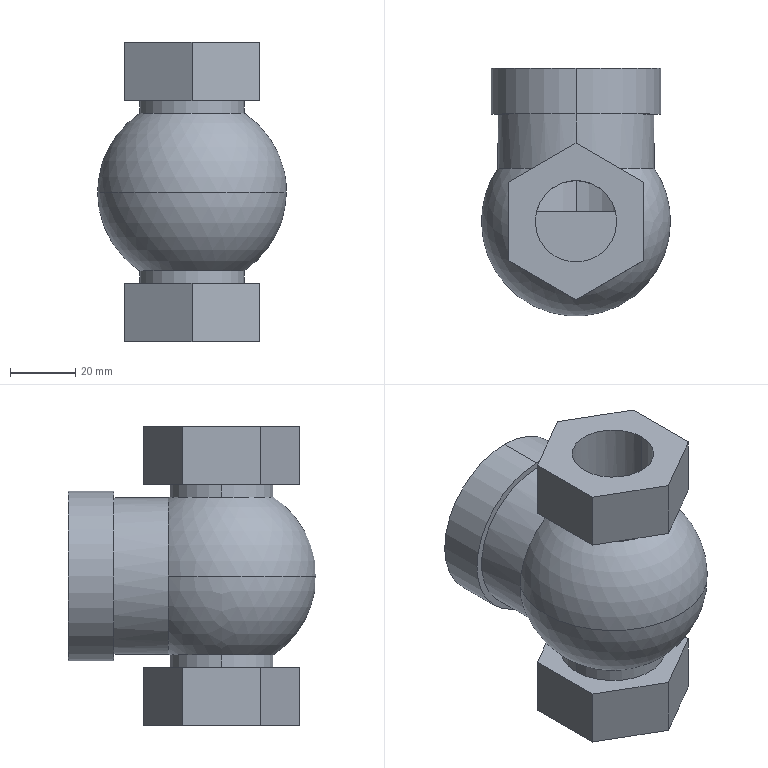Part | SolidWorks | features ICE 8, RevCut 3, MirrorPattern 1, Revolution 1 | 1 solid | 49 faces | box 58 x 76 x 92 mm | volume 132810 mm3 | plane 23 | cylinder 22 | sphere 2 | cone 2 | commonest cylinder face diameters 5 x6 25 x4 32 x4 35 x2 40 x2 48 x2
STEP:
#1=CARTESIAN_POINT('',(0.,-1.,2.5));
#2=VERTEX_POINT('',#1);
#3=CARTESIAN_POINT('',(0.,-1.,-2.5));
#4=VERTEX_POINT('',#3);
#5=CARTESIAN_POINT('',(0.,-1.,0.));
#6=DIRECTION('',(0.,-1.,0.));
#7=DIRECTION('',(0.,0.,1.));
#8=AXIS2_PLACEMENT_3D('',#5,#6,#7);
#9=CIRCLE('',#8,2.5);
#10=EDGE_CURVE('',#2,#4,#9,.T.);
#11=ORIENTED_EDGE('',*,*,#10,.F.);
#12=CARTESIAN_POINT('',(0.,-2.5,2.5));
#13=VERTEX_POINT('',#12);
#14=CARTESIAN_POINT('',(0.,-5.,2.5));
#15=DIRECTION('',(0.,-1.,0.));
#16=VECTOR('',#15,1000.);
#17=LINE('',#14,#16);
#18=EDGE_CURVE('',#2,#13,#17,.T.);
#19=ORIENTED_EDGE('',*,*,#18,.T.);
#20=CARTESIAN_POINT('',(-2.5,-5.,0.));
#21=VERTEX_POINT('',#20);
#22=CARTESIAN_POINT('',(0.,-2.5,2.5));
#23=CARTESIAN_POINT('',(-1.464,-2.5,2.5));
#24=CARTESIAN_POINT('',(-2.5,-3.536,1.464));
#25=CARTESIAN_POINT('',(-2.5,-5.,0.));
#26=(BOUNDED_CURVE()B_SPLINE_CURVE(3,(#22,#23,#24,#25),.UNSPECIFIED.,.F.,.T.)B_SPLINE_CURVE_WITH_KNOTS((4,4),(0.,1.571),.UNSPECIFIED.)CURVE()GEOMETRIC_REPRESENTATION_ITEM()RATIONAL_B_SPLINE_CURVE((1.,0.8047,0.8047,1.))REPRESENTATION_ITEM(''));
#27=EDGE_CURVE('',#13,#21,#26,.T.);
#28=ORIENTED_EDGE('',*,*,#27,.T.);
#29=CARTESIAN_POINT('',(0.,-2.5,-2.5));
#30=VERTEX_POINT('',#29);
#31=CARTESIAN_POINT('',(-2.5,-5.,0.));
#32=CARTESIAN_POINT('',(-2.5,-3.536,-1.464));
#33=CARTESIAN_POINT('',(-1.464,-2.5,-2.5));
#34=CARTESIAN_POINT('',(0.,-2.5,-2.5));
#35=(BOUNDED_CURVE()B_SPLINE_CURVE(3,(#31,#32,#33,#34),.UNSPECIFIED.,.F.,.T.)B_SPLINE_CURVE_WITH_KNOTS((4,4),(1.571,3.142),.UNSPECIFIED.)CURVE()GEOMETRIC_REPRESENTATION_ITEM()RATIONAL_B_SPLINE_CURVE((1.,0.8047,0.8047,1.))REPRESENTATION_ITEM(''));
#36=EDGE_CURVE('',#21,#30,#35,.T.);
#37=ORIENTED_EDGE('',*,*,#36,.T.);
#38=CARTESIAN_POINT('',(0.,-5.,-2.5));
#39=DIRECTION('',(0.,-1.,0.));
#40=VECTOR('',#39,1000.);
#41=LINE('',#38,#40);
#42=EDGE_CURVE('',#4,#30,#41,.T.);
#43=ORIENTED_EDGE('',*,*,#42,.F.);
#44=EDGE_LOOP('',(#11,#19,#28,#37,#43));
#45=FACE_OUTER_BOUND('',#44,.T.);
#46=CARTESIAN_POINT('',(0.,-5.,0.));
#47=DIRECTION('',(0.,-1.,0.));
#48=DIRECTION('',(0.,0.,-1.));
#49=AXIS2_PLACEMENT_3D('',#46,#47,#48);
#50=CYLINDRICAL_SURFACE('',#49,2.5);
#51=ADVANCED_FACE('',(#45),#50,.F.);
#52=CARTESIAN_POINT('',(0.,3.,-17.5));
#53=VERTEX_POINT('',#52);
#54=CARTESIAN_POINT('',(-12.135,3.,12.61));
#55=VERTEX_POINT('',#54);
#56=CARTESIAN_POINT('',(0.,3.,0.));
#57=DIRECTION('',(0.,1.,0.));
#58=DIRECTION('',(0.,0.,1.));
#59=AXIS2_PLACEMENT_3D('',#56,#57,#58);
#60=CIRCLE('',#59,17.5);
#61=EDGE_CURVE('',#53,#55,#60,.T.);
#62=ORIENTED_EDGE('',*,*,#61,.F.);
#63=CARTESIAN_POINT('',(0.,42.,-17.5));
#64=VERTEX_POINT('',#63);
#65=CARTESIAN_POINT('',(0.,3.,-17.5));
#66=DIRECTION('',(0.,1.,0.));
#67=VECTOR('',#66,1000.);
#68=LINE('',#65,#67);
#69=EDGE_CURVE('',#53,#64,#68,.T.);
#70=ORIENTED_EDGE('',*,*,#69,.T.);
#71=CARTESIAN_POINT('',(0.,42.,17.5));
#72=VERTEX_POINT('',#71);
#73=CARTESIAN_POINT('',(0.,42.,0.));
#74=DIRECTION('',(0.,1.,0.));
#75=DIRECTION('',(0.,0.,1.));
#76=AXIS2_PLACEMENT_3D('',#73,#74,#75);
#77=CIRCLE('',#76,17.5);
#78=EDGE_CURVE('',#64,#72,#77,.T.);
#79=ORIENTED_EDGE('',*,*,#78,.T.);
#80=CARTESIAN_POINT('',(0.,12.5,17.5));
#81=VERTEX_POINT('',#80);
#82=CARTESIAN_POINT('',(0.,3.,17.5));
#83=DIRECTION('',(0.,1.,0.));
#84=VECTOR('',#83,1000.);
#85=LINE('',#82,#84);
#86=EDGE_CURVE('',#81,#72,#85,.T.);
#87=ORIENTED_EDGE('',*,*,#86,.F.);
#88=CARTESIAN_POINT('',(-12.135,3.,12.61));
#89=CARTESIAN_POINT('',(-11.963,3.695,12.775));
#90=CARTESIAN_POINT('',(-11.738,4.351,12.984));
#91=CARTESIAN_POINT('',(-11.195,5.602,13.455));
#92=CARTESIAN_POINT('',(-10.877,6.198,13.717));
#93=CARTESIAN_POINT('',(-10.143,7.337,14.268));
#94=CARTESIAN_POINT('',(-9.736,7.868,14.551));
#95=CARTESIAN_POINT('',(-8.842,8.86,15.111));
#96=CARTESIAN_POINT('',(-8.356,9.322,15.388));
#97=CARTESIAN_POINT('',(-7.293,10.175,15.919));
#98=CARTESIAN_POINT('',(-6.728,10.557,16.167));
#99=CARTESIAN_POINT('',(-5.537,11.228,16.613));
#100=CARTESIAN_POINT('',(-4.909,11.518,16.811));
#101=CARTESIAN_POINT('',(-3.911,11.878,17.061));
#102=CARTESIAN_POINT('',(-3.567,11.986,17.136));
#103=CARTESIAN_POINT('',(-2.872,12.171,17.266));
#104=CARTESIAN_POINT('',(-2.522,12.248,17.321));
#105=CARTESIAN_POINT('',(-1.813,12.373,17.409));
#106=CARTESIAN_POINT('',(-1.455,12.42,17.443));
#107=CARTESIAN_POINT('',(-0.733,12.484,17.488));
#108=CARTESIAN_POINT('',(-0.3665,12.5,17.5));
#109=CARTESIAN_POINT('',(0.,12.5,17.5));
#110=B_SPLINE_CURVE_WITH_KNOTS('',3,(#88,#89,#90,#91,#92,#93,#94,#95,#96,#97,#98,#99,#100,#101,#102,#103,#104,#105,#106,#107,#108,#109),.UNSPECIFIED.,.F.,.F.,(4,2,2,2,2,2,2,2,2,2,4),(0.,0.002165,0.00433,0.006494,0.008659,0.01082,0.01299,0.01407,0.01515,0.01624,0.01732),.UNSPECIFIED.);
#111=EDGE_CURVE('',#55,#81,#110,.T.);
#112=ORIENTED_EDGE('',*,*,#111,.F.);
#113=EDGE_LOOP('',(#62,#70,#79,#87,#112));
#114=FACE_OUTER_BOUND('',#113,.T.);
#115=CARTESIAN_POINT('',(0.,3.,0.));
#116=DIRECTION('',(0.,1.,0.));
#117=DIRECTION('',(0.,0.,1.));
#118=AXIS2_PLACEMENT_3D('',#115,#116,#117);
#119=CYLINDRICAL_SURFACE('',#118,17.5);
#120=ADVANCED_FACE('',(#114),#119,.F.);
#121=CARTESIAN_POINT('',(12.5,0.,-21.));
#122=VERTEX_POINT('',#121);
#123=CARTESIAN_POINT('',(-12.5,0.,-21.));
#124=VERTEX_POINT('',#123);
#125=CARTESIAN_POINT('',(0.,0.,-21.));
#126=DIRECTION('',(0.,0.,-1.));
#127=DIRECTION('',(-1.,0.,0.));
#128=AXIS2_PLACEMENT_3D('',#125,#126,#127);
#129=CIRCLE('',#128,12.5);
#130=EDGE_CURVE('',#122,#124,#129,.T.);
#131=ORIENTED_EDGE('',*,*,#130,.F.);
#132=CARTESIAN_POINT('',(12.5,0.,-46.));
#133=VERTEX_POINT('',#132);
#134=CARTESIAN_POINT('',(12.5,0.,-21.));
#135=DIRECTION('',(0.,0.,-1.));
#136=VECTOR('',#135,1000.);
#137=LINE('',#134,#136);
#138=EDGE_CURVE('',#122,#133,#137,.T.);
#139=ORIENTED_EDGE('',*,*,#138,.T.);
#140=CARTESIAN_POINT('',(-12.5,0.,-46.));
#141=VERTEX_POINT('',#140);
#142=CARTESIAN_POINT('',(0.,0.,-46.));
#143=DIRECTION('',(0.,0.,-1.));
#144=DIRECTION('',(-1.,0.,0.));
#145=AXIS2_PLACEMENT_3D('',#142,#143,#144);
#146=CIRCLE('',#145,12.5);
#147=EDGE_CURVE('',#133,#141,#146,.T.);
#148=ORIENTED_EDGE('',*,*,#147,.T.);
#149=CARTESIAN_POINT('',(-12.5,0.,-21.));
#150=DIRECTION('',(0.,0.,-1.));
#151=VECTOR('',#150,1000.);
#152=LINE('',#149,#151);
#153=EDGE_CURVE('',#124,#141,#152,.T.);
#154=ORIENTED_EDGE('',*,*,#153,.F.);
#155=EDGE_LOOP('',(#131,#139,#148,#154));
#156=FACE_OUTER_BOUND('',#155,.T.);
#157=CARTESIAN_POINT('',(0.,0.,-21.));
#158=DIRECTION('',(0.,0.,-1.));
#159=DIRECTION('',(-1.,0.,0.));
#160=AXIS2_PLACEMENT_3D('',#157,#158,#159);
#161=CYLINDRICAL_SURFACE('',#160,12.5);
#162=ADVANCED_FACE('',(#156),#161,.F.);
#163=CARTESIAN_POINT('',(0.,42.,-20.));
#164=VERTEX_POINT('',#163);
#165=CARTESIAN_POINT('',(0.,42.,20.));
#166=VERTEX_POINT('',#165);
#167=CARTESIAN_POINT('',(0.,42.,0.));
#168=DIRECTION('',(0.,1.,0.));
#169=DIRECTION('',(0.,0.,1.));
#170=AXIS2_PLACEMENT_3D('',#167,#168,#169);
#171=CIRCLE('',#170,20.);
#172=EDGE_CURVE('',#164,#166,#171,.T.);
#173=ORIENTED_EDGE('',*,*,#172,.F.);
#174=CARTESIAN_POINT('',(0.,47.,-20.));
#175=VERTEX_POINT('',#174);
#176=CARTESIAN_POINT('',(0.,42.,-20.));
#177=DIRECTION('',(0.,1.,0.));
#178=VECTOR('',#177,1000.);
#179=LINE('',#176,#178);
#180=EDGE_CURVE('',#164,#175,#179,.T.);
#181=ORIENTED_EDGE('',*,*,#180,.T.);
#182=CARTESIAN_POINT('',(0.,47.,20.));
#183=VERTEX_POINT('',#182);
#184=CARTESIAN_POINT('',(0.,47.,0.));
#185=DIRECTION('',(0.,1.,0.));
#186=DIRECTION('',(0.,0.,1.));
#187=AXIS2_PLACEMENT_3D('',#184,#185,#186);
#188=CIRCLE('',#187,20.);
#189=EDGE_CURVE('',#175,#183,#188,.T.);
#190=ORIENTED_EDGE('',*,*,#189,.T.);
#191=CARTESIAN_POINT('',(0.,42.,20.));
#192=DIRECTION('',(0.,1.,0.));
#193=VECTOR('',#192,1000.);
#194=LINE('',#191,#193);
#195=EDGE_CURVE('',#166,#183,#194,.T.);
#196=ORIENTED_EDGE('',*,*,#195,.F.);
#197=EDGE_LOOP('',(#173,#181,#190,#196));
#198=FACE_OUTER_BOUND('',#197,.T.);
#199=CARTESIAN_POINT('',(0.,42.,0.));
#200=DIRECTION('',(0.,1.,0.));
#201=DIRECTION('',(0.,0.,1.));
#202=AXIS2_PLACEMENT_3D('',#199,#200,#201);
#203=CYLINDRICAL_SURFACE('',#202,20.);
#204=ADVANCED_FACE('',(#198),#203,.F.);
#205=CARTESIAN_POINT('',(0.,33.,26.));
#206=VERTEX_POINT('',#205);
#207=CARTESIAN_POINT('',(0.,33.,-26.));
#208=VERTEX_POINT('',#207);
#209=CARTESIAN_POINT('',(0.,33.,0.));
#210=DIRECTION('',(0.,1.,0.));
#211=DIRECTION('',(0.,0.,1.));
#212=AXIS2_PLACEMENT_3D('',#209,#210,#211);
#213=CIRCLE('',#212,26.);
#214=EDGE_CURVE('',#206,#208,#213,.T.);
#215=ORIENTED_EDGE('',*,*,#214,.T.);
#216=CARTESIAN_POINT('',(0.,47.,-26.));
#217=VERTEX_POINT('',#216);
#218=CARTESIAN_POINT('',(0.,33.,-26.));
#219=DIRECTION('',(0.,1.,0.));
#220=VECTOR('',#219,1000.);
#221=LINE('',#218,#220);
#222=EDGE_CURVE('',#208,#217,#221,.T.);
#223=ORIENTED_EDGE('',*,*,#222,.T.);
#224=CARTESIAN_POINT('',(0.,47.,26.));
#225=VERTEX_POINT('',#224);
#226=CARTESIAN_POINT('',(0.,47.,0.));
#227=DIRECTION('',(0.,1.,0.));
#228=DIRECTION('',(0.,0.,1.));
#229=AXIS2_PLACEMENT_3D('',#226,#227,#228);
#230=CIRCLE('',#229,26.);
#231=EDGE_CURVE('',#225,#217,#230,.T.);
#232=ORIENTED_EDGE('',*,*,#231,.F.);
#233=CARTESIAN_POINT('',(0.,33.,26.));
#234=DIRECTION('',(0.,1.,0.));
#235=VECTOR('',#234,1000.);
#236=LINE('',#233,#235);
#237=EDGE_CURVE('',#206,#225,#236,.T.);
#238=ORIENTED_EDGE('',*,*,#237,.F.);
#239=EDGE_LOOP('',(#215,#223,#232,#238));
#240=FACE_OUTER_BOUND('',#239,.T.);
#241=CARTESIAN_POINT('',(0.,33.,0.));
#242=DIRECTION('',(0.,1.,0.));
#243=DIRECTION('',(0.,0.,1.));
#244=AXIS2_PLACEMENT_3D('',#241,#242,#243);
#245=CYLINDRICAL_SURFACE('',#244,26.);
#246=ADVANCED_FACE('',(#240),#245,.T.);
#247=CARTESIAN_POINT('',(0.,33.,24.));
#248=VERTEX_POINT('',#247);
#249=CARTESIAN_POINT('',(0.,33.,-24.));
#250=VERTEX_POINT('',#249);
#251=CARTESIAN_POINT('',(0.,33.,0.));
#252=DIRECTION('',(0.,1.,0.));
#253=DIRECTION('',(0.,0.,1.));
#254=AXIS2_PLACEMENT_3D('',#251,#252,#253);
#255=CIRCLE('',#254,24.);
#256=EDGE_CURVE('',#248,#250,#255,.T.);
#257=ORIENTED_EDGE('',*,*,#256,.F.);
#258=CARTESIAN_POINT('',(0.,16.279,24.));
#259=VERTEX_POINT('',#258);
#260=CARTESIAN_POINT('',(0.,47.,24.));
#261=DIRECTION('',(0.,-1.,0.));
#262=VECTOR('',#261,1000.);
#263=LINE('',#260,#262);
#264=EDGE_CURVE('',#248,#259,#263,.T.);
#265=ORIENTED_EDGE('',*,*,#264,.T.);
#266=CARTESIAN_POINT('',(24.,16.279,0.));
#267=VERTEX_POINT('',#266);
#268=CARTESIAN_POINT('',(0.,16.279,0.));
#269=DIRECTION('',(0.,1.,0.));
#270=DIRECTION('',(0.,0.,-1.));
#271=AXIS2_PLACEMENT_3D('',#268,#269,#270);
#272=CIRCLE('',#271,24.);
#273=EDGE_CURVE('',#259,#267,#272,.T.);
#274=ORIENTED_EDGE('',*,*,#273,.T.);
#275=CARTESIAN_POINT('',(0.,16.279,-24.));
#276=VERTEX_POINT('',#275);
#277=CARTESIAN_POINT('',(0.,16.279,0.));
#278=DIRECTION('',(0.,1.,0.));
#279=DIRECTION('',(0.,0.,-1.));
#280=AXIS2_PLACEMENT_3D('',#277,#278,#279);
#281=CIRCLE('',#280,24.);
#282=EDGE_CURVE('',#267,#276,#281,.T.);
#283=ORIENTED_EDGE('',*,*,#282,.T.);
#284=CARTESIAN_POINT('',(0.,47.,-24.));
#285=DIRECTION('',(0.,-1.,0.));
#286=VECTOR('',#285,1000.);
#287=LINE('',#284,#286);
#288=EDGE_CURVE('',#250,#276,#287,.T.);
#289=ORIENTED_EDGE('',*,*,#288,.F.);
#290=EDGE_LOOP('',(#257,#265,#274,#283,#289));
#291=FACE_OUTER_BOUND('',#290,.T.);
#292=CARTESIAN_POINT('',(0.,47.,0.));
#293=DIRECTION('',(0.,-1.,0.));
#294=DIRECTION('',(0.,0.,-1.));
#295=AXIS2_PLACEMENT_3D('',#292,#293,#294);
#296=CYLINDRICAL_SURFACE('',#295,24.);
#297=ADVANCED_FACE('',(#291),#296,.T.);
#298=CARTESIAN_POINT('',(16.,0.,-24.187));
#299=VERTEX_POINT('',#298);
#300=CARTESIAN_POINT('',(-16.,0.,-24.187));
#301=VERTEX_POINT('',#300);
#302=CARTESIAN_POINT('',(0.,0.,-24.187));
#303=DIRECTION('',(0.,0.,1.));
#304=DIRECTION('',(1.,0.,0.));
#305=AXIS2_PLACEMENT_3D('',#302,#303,#304);
#306=CIRCLE('',#305,16.);
#307=EDGE_CURVE('',#299,#301,#306,.T.);
#308=ORIENTED_EDGE('',*,*,#307,.T.);
#309=CARTESIAN_POINT('',(0.,0.,-24.187));
#310=DIRECTION('',(0.,0.,1.));
#311=DIRECTION('',(1.,0.,0.));
#312=AXIS2_PLACEMENT_3D('',#309,#310,#311);
#313=CIRCLE('',#312,16.);
#314=EDGE_CURVE('',#301,#299,#313,.T.);
#315=ORIENTED_EDGE('',*,*,#314,.T.);
#316=EDGE_LOOP('',(#308,#315));
#317=FACE_BOUND('',#316,.T.);
#318=CARTESIAN_POINT('',(29.,0.,0.));
#319=VERTEX_POINT('',#318);
#320=CARTESIAN_POINT('',(0.,0.,0.));
#321=DIRECTION('',(0.,0.,1.));
#322=DIRECTION('',(1.,0.,0.));
#323=AXIS2_PLACEMENT_3D('',#320,#321,#322);
#324=CIRCLE('',#323,29.);
#325=EDGE_CURVE('',#319,#267,#324,.T.);
#326=ORIENTED_EDGE('',*,*,#325,.F.);
#327=CARTESIAN_POINT('',(-29.,0.,0.));
#328=VERTEX_POINT('',#327);
#329=CARTESIAN_POINT('',(0.,0.,0.));
#330=DIRECTION('',(0.,0.,-1.));
#331=DIRECTION('',(0.,1.,0.));
#332=AXIS2_PLACEMENT_3D('',#329,#330,#331);
#333=CIRCLE('',#332,29.);
#334=EDGE_CURVE('',#319,#328,#333,.T.);
#335=ORIENTED_EDGE('',*,*,#334,.T.);
#336=CARTESIAN_POINT('',(-24.,16.279,0.));
#337=VERTEX_POINT('',#336);
#338=CARTESIAN_POINT('',(0.,0.,0.));
#339=DIRECTION('',(0.,0.,1.));
#340=DIRECTION('',(1.,0.,0.));
#341=AXIS2_PLACEMENT_3D('',#338,#339,#340);
#342=CIRCLE('',#341,29.);
#343=EDGE_CURVE('',#337,#328,#342,.T.);
#344=ORIENTED_EDGE('',*,*,#343,.F.);
#345=CARTESIAN_POINT('',(0.,16.279,0.));
#346=DIRECTION('',(0.,1.,0.));
#347=DIRECTION('',(0.,0.,-1.));
#348=AXIS2_PLACEMENT_3D('',#345,#346,#347);
#349=CIRCLE('',#348,24.);
#350=EDGE_CURVE('',#276,#337,#349,.T.);
#351=ORIENTED_EDGE('',*,*,#350,.F.);
#352=ORIENTED_EDGE('',*,*,#282,.F.);
#353=EDGE_LOOP('',(#326,#335,#344,#351,#352));
#354=FACE_OUTER_BOUND('',#353,.T.);
#355=CARTESIAN_POINT('',(0.,0.,0.));
#356=DIRECTION('',(0.,0.,-1.));
#357=DIRECTION('',(0.,1.,0.));
#358=AXIS2_PLACEMENT_3D('',#355,#356,#357);
#359=SPHERICAL_SURFACE('',#358,29.);
#360=ADVANCED_FACE('',(#317,#354),#359,.T.);
#361=CARTESIAN_POINT('',(16.,0.,28.));
#362=VERTEX_POINT('',#361);
#363=CARTESIAN_POINT('',(-16.,0.,28.));
#364=VERTEX_POINT('',#363);
#365=CARTESIAN_POINT('',(0.,0.,28.));
#366=DIRECTION('',(0.,0.,1.));
#367=DIRECTION('',(1.,0.,0.));
#368=AXIS2_PLACEMENT_3D('',#365,#366,#367);
#369=CIRCLE('',#368,16.);
#370=EDGE_CURVE('',#362,#364,#369,.T.);
#371=ORIENTED_EDGE('',*,*,#370,.F.);
#372=CARTESIAN_POINT('',(16.,0.,24.187));
#373=VERTEX_POINT('',#372);
#374=CARTESIAN_POINT('',(16.,0.,46.));
#375=DIRECTION('',(0.,0.,-1.));
#376=VECTOR('',#375,1000.);
#377=LINE('',#374,#376);
#378=EDGE_CURVE('',#362,#373,#377,.T.);
#379=ORIENTED_EDGE('',*,*,#378,.T.);
#380=CARTESIAN_POINT('',(-16.,0.,24.187));
#381=VERTEX_POINT('',#380);
#382=CARTESIAN_POINT('',(0.,0.,24.187));
#383=DIRECTION('',(0.,0.,1.));
#384=DIRECTION('',(-1.,0.,0.));
#385=AXIS2_PLACEMENT_3D('',#382,#383,#384);
#386=CIRCLE('',#385,16.);
#387=EDGE_CURVE('',#373,#381,#386,.T.);
#388=ORIENTED_EDGE('',*,*,#387,.T.);
#389=CARTESIAN_POINT('',(-16.,0.,46.));
#390=DIRECTION('',(0.,0.,-1.));
#391=VECTOR('',#390,1000.);
#392=LINE('',#389,#391);
#393=EDGE_CURVE('',#364,#381,#392,.T.);
#394=ORIENTED_EDGE('',*,*,#393,.F.);
#395=EDGE_LOOP('',(#371,#379,#388,#394));
#396=FACE_OUTER_BOUND('',#395,.T.);
#397=CARTESIAN_POINT('',(0.,0.,46.));
#398=DIRECTION('',(0.,0.,-1.));
#399=DIRECTION('',(-1.,0.,0.));
#400=AXIS2_PLACEMENT_3D('',#397,#398,#399);
#401=CYLINDRICAL_SURFACE('',#400,16.);
#402=ADVANCED_FACE('',(#396),#401,.T.);
#403=CARTESIAN_POINT('',(16.,0.,-28.));
#404=VERTEX_POINT('',#403);
#405=CARTESIAN_POINT('',(-16.,0.,-28.));
#406=VERTEX_POINT('',#405);
#407=CARTESIAN_POINT('',(0.,0.,-28.));
#408=DIRECTION('',(0.,0.,1.));
#409=DIRECTION('',(-1.,0.,0.));
#410=AXIS2_PLACEMENT_3D('',#407,#408,#409);
#411=CIRCLE('',#410,16.);
#412=EDGE_CURVE('',#404,#406,#411,.T.);
#413=ORIENTED_EDGE('',*,*,#412,.T.);
#414=CARTESIAN_POINT('',(-16.,0.,-46.));
#415=DIRECTION('',(0.,0.,1.));
#416=VECTOR('',#415,1000.);
#417=LINE('',#414,#416);
#418=EDGE_CURVE('',#406,#301,#417,.T.);
#419=ORIENTED_EDGE('',*,*,#418,.T.);
#420=ORIENTED_EDGE('',*,*,#307,.F.);
#421=CARTESIAN_POINT('',(16.,0.,-46.));
#422=DIRECTION('',(0.,0.,1.));
#423=VECTOR('',#422,1000.);
#424=LINE('',#421,#423);
#425=EDGE_CURVE('',#404,#299,#424,.T.);
#426=ORIENTED_EDGE('',*,*,#425,.F.);
#427=EDGE_LOOP('',(#413,#419,#420,#426));
#428=FACE_OUTER_BOUND('',#427,.T.);
#429=CARTESIAN_POINT('',(0.,0.,-46.));
#430=DIRECTION('',(0.,0.,1.));
#431=DIRECTION('',(1.,0.,0.));
#432=AXIS2_PLACEMENT_3D('',#429,#430,#431);
#433=CYLINDRICAL_SURFACE('',#432,16.);
#434=ADVANCED_FACE('',(#428),#433,.T.);
#435=CARTESIAN_POINT('',(-12.5,0.,12.));
#436=VERTEX_POINT('',#435);
#437=CARTESIAN_POINT('',(12.5,0.,12.));
#438=VERTEX_POINT('',#437);
#439=CARTESIAN_POINT('',(0.,0.,12.));
#440=DIRECTION('',(0.,0.,1.));
#441=DIRECTION('',(1.,0.,0.));
#442=AXIS2_PLACEMENT_3D('',#439,#440,#441);
#443=CIRCLE('',#442,12.5);
#444=EDGE_CURVE('',#436,#438,#443,.T.);
#445=ORIENTED_EDGE('',*,*,#444,.F.);
#446=CARTESIAN_POINT('',(-12.5,0.,46.));
#447=VERTEX_POINT('',#446);
#448=CARTESIAN_POINT('',(-12.5,0.,12.));
#449=DIRECTION('',(0.,0.,1.));
#450=VECTOR('',#449,1000.);
#451=LINE('',#448,#450);
#452=EDGE_CURVE('',#436,#447,#451,.T.);
#453=ORIENTED_EDGE('',*,*,#452,.T.);
#454=CARTESIAN_POINT('',(12.5,0.,46.));
#455=VERTEX_POINT('',#454);
#456=CARTESIAN_POINT('',(0.,0.,46.));
#457=DIRECTION('',(0.,0.,1.));
#458=DIRECTION('',(1.,0.,0.));
#459=AXIS2_PLACEMENT_3D('',#456,#457,#458);
#460=CIRCLE('',#459,12.5);
#461=EDGE_CURVE('',#447,#455,#460,.T.);
#462=ORIENTED_EDGE('',*,*,#461,.T.);
#463=CARTESIAN_POINT('',(12.5,0.,12.));
#464=DIRECTION('',(0.,0.,1.));
#465=VECTOR('',#464,1000.);
#466=LINE('',#463,#465);
#467=EDGE_CURVE('',#438,#455,#466,.T.);
#468=ORIENTED_EDGE('',*,*,#467,.F.);
#469=EDGE_LOOP('',(#445,#453,#462,#468));
#470=FACE_OUTER_BOUND('',#469,.T.);
#471=CARTESIAN_POINT('',(0.,0.,12.));
#472=DIRECTION('',(0.,0.,1.));
#473=DIRECTION('',(1.,0.,0.));
#474=AXIS2_PLACEMENT_3D('',#471,#472,#473);
#475=CYLINDRICAL_SURFACE('',#474,12.5);
#476=ADVANCED_FACE('',(#470),#475,.F.);
#477=CARTESIAN_POINT('',(2.5,-5.,-21.));
#478=VERTEX_POINT('',#477);
#479=CARTESIAN_POINT('',(-2.5,-5.,-21.));
#480=VERTEX_POINT('',#479);
#481=CARTESIAN_POINT('',(0.,-5.,-21.));
#482=DIRECTION('',(0.,0.,-1.));
#483=DIRECTION('',(-1.,0.,0.));
#484=AXIS2_PLACEMENT_3D('',#481,#482,#483);
#485=CIRCLE('',#484,2.5);
#486=EDGE_CURVE('',#478,#480,#485,.T.);
#487=ORIENTED_EDGE('',*,*,#486,.T.);
#488=CARTESIAN_POINT('',(-2.5,-5.,4.897));
#489=DIRECTION('',(0.,0.,1.));
#490=VECTOR('',#489,1000.);
#491=LINE('',#488,#490);
#492=EDGE_CURVE('',#480,#21,#491,.T.);
#493=ORIENTED_EDGE('',*,*,#492,.T.);
#494=CARTESIAN_POINT('',(-2.5,-5.,2.5));
#495=VERTEX_POINT('',#494);
#496=CARTESIAN_POINT('',(-2.5,-5.,4.897));
#497=DIRECTION('',(0.,0.,1.));
#498=VECTOR('',#497,1000.);
#499=LINE('',#496,#498);
#500=EDGE_CURVE('',#21,#495,#499,.T.);
#501=ORIENTED_EDGE('',*,*,#500,.T.);
#502=CARTESIAN_POINT('',(2.5,-5.,2.5));
#503=VERTEX_POINT('',#502);
#504=CARTESIAN_POINT('',(0.,-5.,2.5));
#505=DIRECTION('',(0.,0.,1.));
#506=DIRECTION('',(1.,0.,0.));
#507=AXIS2_PLACEMENT_3D('',#504,#505,#506);
#508=CIRCLE('',#507,2.5);
#509=EDGE_CURVE('',#495,#503,#508,.T.);
#510=ORIENTED_EDGE('',*,*,#509,.T.);
#511=CARTESIAN_POINT('',(2.5,-5.,0.));
#512=VERTEX_POINT('',#511);
#513=CARTESIAN_POINT('',(2.5,-5.,4.897));
#514=DIRECTION('',(0.,0.,1.));
#515=VECTOR('',#514,1000.);
#516=LINE('',#513,#515);
#517=EDGE_CURVE('',#512,#503,#516,.T.);
#518=ORIENTED_EDGE('',*,*,#517,.F.);
#519=CARTESIAN_POINT('',(2.5,-5.,4.897));
#520=DIRECTION('',(0.,0.,1.));
#521=VECTOR('',#520,1000.);
#522=LINE('',#519,#521);
#523=EDGE_CURVE('',#478,#512,#522,.T.);
#524=ORIENTED_EDGE('',*,*,#523,.F.);
#525=EDGE_LOOP('',(#487,#493,#501,#510,#518,#524));
#526=FACE_OUTER_BOUND('',#525,.T.);
#527=CARTESIAN_POINT('',(0.,-5.,4.897));
#528=DIRECTION('',(0.,0.,1.));
#529=DIRECTION('',(1.,0.,0.));
#530=AXIS2_PLACEMENT_3D('',#527,#528,#529);
#531=CYLINDRICAL_SURFACE('',#530,2.5);
#532=ADVANCED_FACE('',(#526),#531,.F.);
#533=ORIENTED_EDGE('',*,*,#492,.F.);
#534=CARTESIAN_POINT('',(0.,-5.,-21.));
#535=DIRECTION('',(0.,0.,-1.));
#536=DIRECTION('',(-1.,0.,0.));
#537=AXIS2_PLACEMENT_3D('',#534,#535,#536);
#538=CIRCLE('',#537,2.5);
#539=EDGE_CURVE('',#480,#478,#538,.T.);
#540=ORIENTED_EDGE('',*,*,#539,.T.);
#541=ORIENTED_EDGE('',*,*,#523,.T.);
#542=CARTESIAN_POINT('',(0.,-2.5,-2.5));
#543=CARTESIAN_POINT('',(1.464,-2.5,-2.5));
#544=CARTESIAN_POINT('',(2.5,-3.536,-1.464));
#545=CARTESIAN_POINT('',(2.5,-5.,0.));
#546=(BOUNDED_CURVE()B_SPLINE_CURVE(3,(#542,#543,#544,#545),.UNSPECIFIED.,.F.,.T.)B_SPLINE_CURVE_WITH_KNOTS((4,4),(3.142,4.712),.UNSPECIFIED.)CURVE()GEOMETRIC_REPRESENTATION_ITEM()RATIONAL_B_SPLINE_CURVE((1.,0.8047,0.8047,1.))REPRESENTATION_ITEM(''));
#547=EDGE_CURVE('',#30,#512,#546,.T.);
#548=ORIENTED_EDGE('',*,*,#547,.F.);
#549=ORIENTED_EDGE('',*,*,#36,.F.);
#550=EDGE_LOOP('',(#533,#540,#541,#548,#549));
#551=FACE_OUTER_BOUND('',#550,.T.);
#552=CARTESIAN_POINT('',(0.,-5.,4.897));
#553=DIRECTION('',(0.,0.,1.));
#554=DIRECTION('',(1.,0.,0.));
#555=AXIS2_PLACEMENT_3D('',#552,#553,#554);
#556=CYLINDRICAL_SURFACE('',#555,2.5);
#557=ADVANCED_FACE('',(#551),#556,.F.);
#558=CARTESIAN_POINT('',(2.5,-5.,0.));
#559=CARTESIAN_POINT('',(2.5,-3.536,1.464));
#560=CARTESIAN_POINT('',(1.464,-2.5,2.5));
#561=CARTESIAN_POINT('',(0.,-2.5,2.5));
#562=(BOUNDED_CURVE()B_SPLINE_CURVE(3,(#558,#559,#560,#561),.UNSPECIFIED.,.F.,.T.)B_SPLINE_CURVE_WITH_KNOTS((4,4),(4.712,6.283),.UNSPECIFIED.)CURVE()GEOMETRIC_REPRESENTATION_ITEM()RATIONAL_B_SPLINE_CURVE((1.,0.8047,0.8047,1.))REPRESENTATION_ITEM(''));
#563=EDGE_CURVE('',#512,#13,#562,.T.);
#564=ORIENTED_EDGE('',*,*,#563,.F.);
#565=ORIENTED_EDGE('',*,*,#517,.T.);
#566=CARTESIAN_POINT('',(0.,-5.,2.5));
#567=DIRECTION('',(0.,0.,1.));
#568=DIRECTION('',(1.,0.,0.));
#569=AXIS2_PLACEMENT_3D('',#566,#567,#568);
#570=CIRCLE('',#569,2.5);
#571=EDGE_CURVE('',#503,#13,#570,.T.);
#572=ORIENTED_EDGE('',*,*,#571,.T.);
#573=EDGE_LOOP('',(#564,#565,#572));
#574=FACE_OUTER_BOUND('',#573,.T.);
#575=CARTESIAN_POINT('',(0.,-5.,4.897));
#576=DIRECTION('',(0.,0.,1.));
#577=DIRECTION('',(1.,0.,0.));
#578=AXIS2_PLACEMENT_3D('',#575,#576,#577);
#579=CYLINDRICAL_SURFACE('',#578,2.5);
#580=ADVANCED_FACE('',(#574),#579,.F.);
#581=ORIENTED_EDGE('',*,*,#10,.T.);
#582=CARTESIAN_POINT('',(0.,3.,-6.5));
#583=VERTEX_POINT('',#582);
#584=CARTESIAN_POINT('',(0.,3.,-6.5));
#585=DIRECTION('',(0.,0.7071,-0.7071));
#586=VECTOR('',#585,1000.);
#587=LINE('',#584,#586);
#588=EDGE_CURVE('',#4,#583,#587,.T.);
#589=ORIENTED_EDGE('',*,*,#588,.T.);
#590=CARTESIAN_POINT('',(0.,3.,6.5));
#591=VERTEX_POINT('',#590);
#592=CARTESIAN_POINT('',(0.,3.,0.));
#593=DIRECTION('',(0.,-1.,0.));
#594=DIRECTION('',(0.,0.,-1.));
#595=AXIS2_PLACEMENT_3D('',#592,#593,#594);
#596=CIRCLE('',#595,6.5);
#597=EDGE_CURVE('',#591,#583,#596,.T.);
#598=ORIENTED_EDGE('',*,*,#597,.F.);
#599=CARTESIAN_POINT('',(0.,3.,6.5));
#600=DIRECTION('',(0.,0.7071,0.7071));
#601=VECTOR('',#600,1000.);
#602=LINE('',#599,#601);
#603=EDGE_CURVE('',#2,#591,#602,.T.);
#604=ORIENTED_EDGE('',*,*,#603,.F.);
#605=EDGE_LOOP('',(#581,#589,#598,#604));
#606=FACE_OUTER_BOUND('',#605,.T.);
#607=CARTESIAN_POINT('',(0.,3.,0.));
#608=DIRECTION('',(0.,1.,0.));
#609=DIRECTION('',(0.,0.,1.));
#610=AXIS2_PLACEMENT_3D('',#607,#608,#609);
#611=CONICAL_SURFACE('',#610,6.5,0.7854);
#612=ADVANCED_FACE('',(#606),#611,.F.);
#613=ORIENTED_EDGE('',*,*,#588,.F.);
#614=CARTESIAN_POINT('',(0.,-1.,0.));
#615=DIRECTION('',(0.,-1.,0.));
#616=DIRECTION('',(0.,0.,1.));
#617=AXIS2_PLACEMENT_3D('',#614,#615,#616);
#618=CIRCLE('',#617,2.5);
#619=EDGE_CURVE('',#4,#2,#618,.T.);
#620=ORIENTED_EDGE('',*,*,#619,.T.);
#621=ORIENTED_EDGE('',*,*,#603,.T.);
#622=CARTESIAN_POINT('',(0.,3.,0.));
#623=DIRECTION('',(0.,-1.,0.));
#624=DIRECTION('',(0.,0.,-1.));
#625=AXIS2_PLACEMENT_3D('',#622,#623,#624);
#626=CIRCLE('',#625,6.5);
#627=EDGE_CURVE('',#583,#591,#626,.T.);
#628=ORIENTED_EDGE('',*,*,#627,.F.);
#629=EDGE_LOOP('',(#613,#620,#621,#628));
#630=FACE_OUTER_BOUND('',#629,.T.);
#631=CARTESIAN_POINT('',(0.,3.,0.));
#632=DIRECTION('',(0.,1.,0.));
#633=DIRECTION('',(0.,0.,1.));
#634=AXIS2_PLACEMENT_3D('',#631,#632,#633);
#635=CONICAL_SURFACE('',#634,6.5,0.7854);
#636=ADVANCED_FACE('',(#630),#635,.F.);
#637=ORIENTED_EDGE('',*,*,#500,.F.);
#638=ORIENTED_EDGE('',*,*,#27,.F.);
#639=CARTESIAN_POINT('',(0.,-5.,2.5));
#640=DIRECTION('',(0.,0.,1.));
#641=DIRECTION('',(1.,0.,0.));
#642=AXIS2_PLACEMENT_3D('',#639,#640,#641);
#643=CIRCLE('',#642,2.5);
#644=EDGE_CURVE('',#13,#495,#643,.T.);
#645=ORIENTED_EDGE('',*,*,#644,.T.);
#646=EDGE_LOOP('',(#637,#638,#645));
#647=FACE_OUTER_BOUND('',#646,.T.);
#648=CARTESIAN_POINT('',(0.,-5.,4.897));
#649=DIRECTION('',(0.,0.,1.));
#650=DIRECTION('',(1.,0.,0.));
#651=AXIS2_PLACEMENT_3D('',#648,#649,#650);
#652=CYLINDRICAL_SURFACE('',#651,2.5);
#653=ADVANCED_FACE('',(#647),#652,.F.);
#654=CARTESIAN_POINT('',(-12.135,3.,12.));
#655=VERTEX_POINT('',#654);
#656=CARTESIAN_POINT('',(-12.135,3.,12.));
#657=DIRECTION('',(0.,0.,-1.));
#658=VECTOR('',#657,1000.);
#659=LINE('',#656,#658);
#660=EDGE_CURVE('',#55,#655,#659,.T.);
#661=ORIENTED_EDGE('',*,*,#660,.T.);
#662=CARTESIAN_POINT('',(12.135,3.,12.));
#663=VERTEX_POINT('',#662);
#664=CARTESIAN_POINT('',(0.,3.,12.));
#665=DIRECTION('',(-1.,0.,0.));
#666=VECTOR('',#665,1000.);
#667=LINE('',#664,#666);
#668=EDGE_CURVE('',#663,#655,#667,.T.);
#669=ORIENTED_EDGE('',*,*,#668,.F.);
#670=CARTESIAN_POINT('',(12.135,3.,12.61));
#671=VERTEX_POINT('',#670);
#672=CARTESIAN_POINT('',(12.135,3.,12.));
#673=DIRECTION('',(0.,0.,1.));
#674=VECTOR('',#673,1000.);
#675=LINE('',#672,#674);
#676=EDGE_CURVE('',#663,#671,#675,.T.);
#677=ORIENTED_EDGE('',*,*,#676,.T.);
#678=CARTESIAN_POINT('',(0.,3.,0.));
#679=DIRECTION('',(0.,1.,0.));
#680=DIRECTION('',(0.,0.,1.));
#681=AXIS2_PLACEMENT_3D('',#678,#679,#680);
#682=CIRCLE('',#681,17.5);
#683=EDGE_CURVE('',#671,#53,#682,.T.);
#684=ORIENTED_EDGE('',*,*,#683,.T.);
#685=ORIENTED_EDGE('',*,*,#61,.T.);
#686=EDGE_LOOP('',(#661,#669,#677,#684,#685));
#687=FACE_OUTER_BOUND('',#686,.T.);
#688=ORIENTED_EDGE('',*,*,#597,.T.);
#689=ORIENTED_EDGE('',*,*,#627,.T.);
#690=EDGE_LOOP('',(#688,#689));
#691=FACE_BOUND('',#690,.T.);
#692=CARTESIAN_POINT('',(0.,3.,0.));
#693=DIRECTION('',(0.,1.,0.));
#694=DIRECTION('',(0.,0.,1.));
#695=AXIS2_PLACEMENT_3D('',#692,#693,#694);
#696=PLANE('',#695);
#697=ADVANCED_FACE('',(#687,#691),#696,.T.);
#698=ORIENTED_EDGE('',*,*,#452,.F.);
#699=CARTESIAN_POINT('',(0.,0.,12.));
#700=DIRECTION('',(0.,0.,1.));
#701=DIRECTION('',(1.,0.,0.));
#702=AXIS2_PLACEMENT_3D('',#699,#700,#701);
#703=CIRCLE('',#702,12.5);
#704=EDGE_CURVE('',#655,#436,#703,.T.);
#705=ORIENTED_EDGE('',*,*,#704,.F.);
#706=ORIENTED_EDGE('',*,*,#660,.F.);
#707=ORIENTED_EDGE('',*,*,#111,.T.);
#708=CARTESIAN_POINT('',(0.,12.5,17.5));
#709=CARTESIAN_POINT('',(0.7305,12.5,17.5));
#710=CARTESIAN_POINT('',(1.449,12.436,17.454));
#711=CARTESIAN_POINT('',(2.862,12.189,17.279));
#712=CARTESIAN_POINT('',(3.564,12.002,17.147));
#713=CARTESIAN_POINT('',(4.892,11.525,16.816));
#714=CARTESIAN_POINT('',(5.525,11.234,16.618));
#715=CARTESIAN_POINT('',(6.43,10.725,16.279));
#716=CARTESIAN_POINT('',(6.724,10.543,16.159));
#717=CARTESIAN_POINT('',(7.29,10.16,15.912));
#718=CARTESIAN_POINT('',(7.562,9.959,15.784));
#719=CARTESIAN_POINT('',(8.351,9.326,15.39));
#720=CARTESIAN_POINT('',(8.839,8.865,15.113));
#721=CARTESIAN_POINT('',(9.739,7.864,14.549));
#722=CARTESIAN_POINT('',(10.144,7.335,14.267));
#723=CARTESIAN_POINT('',(10.867,6.213,13.724));
#724=CARTESIAN_POINT('',(11.187,5.62,13.462));
#725=CARTESIAN_POINT('',(11.599,4.672,13.105));
#726=CARTESIAN_POINT('',(11.725,4.347,12.992));
#727=CARTESIAN_POINT('',(11.95,3.684,12.786));
#728=CARTESIAN_POINT('',(12.049,3.346,12.692));
#729=CARTESIAN_POINT('',(12.135,3.,12.61));
#730=B_SPLINE_CURVE_WITH_KNOTS('',3,(#708,#709,#710,#711,#712,#713,#714,#715,#716,#717,#718,#719,#720,#721,#722,#723,#724,#725,#726,#727,#728,#729),.UNSPECIFIED.,.F.,.F.,(4,2,2,2,2,2,2,2,2,2,4),(0.01732,0.01948,0.02163,0.02379,0.02487,0.02595,0.0281,0.03026,0.03242,0.0335,0.03458),.UNSPECIFIED.);
#731=EDGE_CURVE('',#81,#671,#730,.T.);
#732=ORIENTED_EDGE('',*,*,#731,.T.);
#733=ORIENTED_EDGE('',*,*,#676,.F.);
#734=CARTESIAN_POINT('',(0.,0.,12.));
#735=DIRECTION('',(0.,0.,1.));
#736=DIRECTION('',(1.,0.,0.));
#737=AXIS2_PLACEMENT_3D('',#734,#735,#736);
#738=CIRCLE('',#737,12.5);
#739=EDGE_CURVE('',#438,#663,#738,.T.);
#740=ORIENTED_EDGE('',*,*,#739,.F.);
#741=ORIENTED_EDGE('',*,*,#467,.T.);
#742=CARTESIAN_POINT('',(0.,0.,46.));
#743=DIRECTION('',(0.,0.,1.));
#744=DIRECTION('',(1.,0.,0.));
#745=AXIS2_PLACEMENT_3D('',#742,#743,#744);
#746=CIRCLE('',#745,12.5);
#747=EDGE_CURVE('',#455,#447,#746,.T.);
#748=ORIENTED_EDGE('',*,*,#747,.T.);
#749=EDGE_LOOP('',(#698,#705,#706,#707,#732,#733,#740,#741,#748));
#750=FACE_OUTER_BOUND('',#749,.T.);
#751=CARTESIAN_POINT('',(0.,0.,12.));
#752=DIRECTION('',(0.,0.,1.));
#753=DIRECTION('',(1.,0.,0.));
#754=AXIS2_PLACEMENT_3D('',#751,#752,#753);
#755=CYLINDRICAL_SURFACE('',#754,12.5);
#756=ADVANCED_FACE('',(#750),#755,.F.);
#757=ORIENTED_EDGE('',*,*,#704,.T.);
#758=ORIENTED_EDGE('',*,*,#444,.T.);
#759=ORIENTED_EDGE('',*,*,#739,.T.);
#760=ORIENTED_EDGE('',*,*,#668,.T.);
#761=EDGE_LOOP('',(#757,#758,#759,#760));
#762=FACE_OUTER_BOUND('',#761,.T.);
#763=CARTESIAN_POINT('',(0.,0.,12.));
#764=DIRECTION('',(0.,0.,1.));
#765=DIRECTION('',(1.,0.,0.));
#766=AXIS2_PLACEMENT_3D('',#763,#764,#765);
#767=PLANE('',#766);
#768=ADVANCED_FACE('',(#762),#767,.T.);
#769=ORIENTED_EDGE('',*,*,#418,.F.);
#770=CARTESIAN_POINT('',(0.,0.,-28.));
#771=DIRECTION('',(0.,0.,1.));
#772=DIRECTION('',(-1.,0.,0.));
#773=AXIS2_PLACEMENT_3D('',#770,#771,#772);
#774=CIRCLE('',#773,16.);
#775=EDGE_CURVE('',#406,#404,#774,.T.);
#776=ORIENTED_EDGE('',*,*,#775,.T.);
#777=ORIENTED_EDGE('',*,*,#425,.T.);
#778=ORIENTED_EDGE('',*,*,#314,.F.);
#779=EDGE_LOOP('',(#769,#776,#777,#778));
#780=FACE_OUTER_BOUND('',#779,.T.);
#781=CARTESIAN_POINT('',(0.,0.,-46.));
#782=DIRECTION('',(0.,0.,1.));
#783=DIRECTION('',(1.,0.,0.));
#784=AXIS2_PLACEMENT_3D('',#781,#782,#783);
#785=CYLINDRICAL_SURFACE('',#784,16.);
#786=ADVANCED_FACE('',(#780),#785,.T.);
#787=ORIENTED_EDGE('',*,*,#378,.F.);
#788=CARTESIAN_POINT('',(0.,0.,28.));
#789=DIRECTION('',(0.,0.,1.));
#790=DIRECTION('',(1.,0.,0.));
#791=AXIS2_PLACEMENT_3D('',#788,#789,#790);
#792=CIRCLE('',#791,16.);
#793=EDGE_CURVE('',#364,#362,#792,.T.);
#794=ORIENTED_EDGE('',*,*,#793,.F.);
#795=ORIENTED_EDGE('',*,*,#393,.T.);
#796=CARTESIAN_POINT('',(0.,0.,24.187));
#797=DIRECTION('',(0.,0.,1.));
#798=DIRECTION('',(-1.,0.,0.));
#799=AXIS2_PLACEMENT_3D('',#796,#797,#798);
#800=CIRCLE('',#799,16.);
#801=EDGE_CURVE('',#381,#373,#800,.T.);
#802=ORIENTED_EDGE('',*,*,#801,.T.);
#803=EDGE_LOOP('',(#787,#794,#795,#802));
#804=FACE_OUTER_BOUND('',#803,.T.);
#805=CARTESIAN_POINT('',(0.,0.,46.));
#806=DIRECTION('',(0.,0.,-1.));
#807=DIRECTION('',(-1.,0.,0.));
#808=AXIS2_PLACEMENT_3D('',#805,#806,#807);
#809=CYLINDRICAL_SURFACE('',#808,16.);
#810=ADVANCED_FACE('',(#804),#809,.T.);
#811=ORIENTED_EDGE('',*,*,#334,.F.);
#812=ORIENTED_EDGE('',*,*,#325,.T.);
#813=ORIENTED_EDGE('',*,*,#273,.F.);
#814=CARTESIAN_POINT('',(0.,16.279,0.));
#815=DIRECTION('',(0.,1.,0.));
#816=DIRECTION('',(0.,0.,-1.));
#817=AXIS2_PLACEMENT_3D('',#814,#815,#816);
#818=CIRCLE('',#817,24.);
#819=EDGE_CURVE('',#337,#259,#818,.T.);
#820=ORIENTED_EDGE('',*,*,#819,.F.);
#821=ORIENTED_EDGE('',*,*,#343,.T.);
#822=EDGE_LOOP('',(#811,#812,#813,#820,#821));
#823=FACE_OUTER_BOUND('',#822,.T.);
#824=ORIENTED_EDGE('',*,*,#801,.F.);
#825=ORIENTED_EDGE('',*,*,#387,.F.);
#826=EDGE_LOOP('',(#824,#825));
#827=FACE_BOUND('',#826,.T.);
#828=CARTESIAN_POINT('',(0.,0.,0.));
#829=DIRECTION('',(0.,0.,-1.));
#830=DIRECTION('',(0.,1.,0.));
#831=AXIS2_PLACEMENT_3D('',#828,#829,#830);
#832=SPHERICAL_SURFACE('',#831,29.);
#833=ADVANCED_FACE('',(#823,#827),#832,.T.);
#834=ORIENTED_EDGE('',*,*,#264,.F.);
#835=CARTESIAN_POINT('',(0.,33.,0.));
#836=DIRECTION('',(0.,1.,0.));
#837=DIRECTION('',(0.,0.,1.));
#838=AXIS2_PLACEMENT_3D('',#835,#836,#837);
#839=CIRCLE('',#838,24.);
#840=EDGE_CURVE('',#250,#248,#839,.T.);
#841=ORIENTED_EDGE('',*,*,#840,.F.);
#842=ORIENTED_EDGE('',*,*,#288,.T.);
#843=ORIENTED_EDGE('',*,*,#350,.T.);
#844=ORIENTED_EDGE('',*,*,#819,.T.);
#845=EDGE_LOOP('',(#834,#841,#842,#843,#844));
#846=FACE_OUTER_BOUND('',#845,.T.);
#847=CARTESIAN_POINT('',(0.,47.,0.));
#848=DIRECTION('',(0.,-1.,0.));
#849=DIRECTION('',(0.,0.,-1.));
#850=AXIS2_PLACEMENT_3D('',#847,#848,#849);
#851=CYLINDRICAL_SURFACE('',#850,24.);
#852=ADVANCED_FACE('',(#846),#851,.T.);
#853=ORIENTED_EDGE('',*,*,#214,.F.);
#854=CARTESIAN_POINT('',(0.,33.,0.));
#855=DIRECTION('',(0.,1.,0.));
#856=DIRECTION('',(0.,0.,1.));
#857=AXIS2_PLACEMENT_3D('',#854,#855,#856);
#858=CIRCLE('',#857,26.);
#859=EDGE_CURVE('',#208,#206,#858,.T.);
#860=ORIENTED_EDGE('',*,*,#859,.F.);
#861=EDGE_LOOP('',(#853,#860));
#862=FACE_OUTER_BOUND('',#861,.T.);
#863=ORIENTED_EDGE('',*,*,#840,.T.);
#864=ORIENTED_EDGE('',*,*,#256,.T.);
#865=EDGE_LOOP('',(#863,#864));
#866=FACE_BOUND('',#865,.T.);
#867=CARTESIAN_POINT('',(0.,33.,0.));
#868=DIRECTION('',(0.,1.,0.));
#869=DIRECTION('',(0.,0.,1.));
#870=AXIS2_PLACEMENT_3D('',#867,#868,#869);
#871=PLANE('',#870);
#872=ADVANCED_FACE('',(#862,#866),#871,.F.);
#873=ORIENTED_EDGE('',*,*,#222,.F.);
#874=ORIENTED_EDGE('',*,*,#859,.T.);
#875=ORIENTED_EDGE('',*,*,#237,.T.);
#876=CARTESIAN_POINT('',(0.,47.,0.));
#877=DIRECTION('',(0.,1.,0.));
#878=DIRECTION('',(0.,0.,1.));
#879=AXIS2_PLACEMENT_3D('',#876,#877,#878);
#880=CIRCLE('',#879,26.);
#881=EDGE_CURVE('',#217,#225,#880,.T.);
#882=ORIENTED_EDGE('',*,*,#881,.F.);
#883=EDGE_LOOP('',(#873,#874,#875,#882));
#884=FACE_OUTER_BOUND('',#883,.T.);
#885=CARTESIAN_POINT('',(0.,33.,0.));
#886=DIRECTION('',(0.,1.,0.));
#887=DIRECTION('',(0.,0.,1.));
#888=AXIS2_PLACEMENT_3D('',#885,#886,#887);
#889=CYLINDRICAL_SURFACE('',#888,26.);
#890=ADVANCED_FACE('',(#884),#889,.T.);
#891=CARTESIAN_POINT('',(0.,47.,0.));
#892=DIRECTION('',(0.,1.,0.));
#893=DIRECTION('',(0.,0.,1.));
#894=AXIS2_PLACEMENT_3D('',#891,#892,#893);
#895=CIRCLE('',#894,20.);
#896=EDGE_CURVE('',#183,#175,#895,.T.);
#897=ORIENTED_EDGE('',*,*,#896,.F.);
#898=ORIENTED_EDGE('',*,*,#189,.F.);
#899=EDGE_LOOP('',(#897,#898));
#900=FACE_BOUND('',#899,.T.);
#901=ORIENTED_EDGE('',*,*,#231,.T.);
#902=ORIENTED_EDGE('',*,*,#881,.T.);
#903=EDGE_LOOP('',(#901,#902));
#904=FACE_OUTER_BOUND('',#903,.T.);
#905=CARTESIAN_POINT('',(0.,47.,0.));
#906=DIRECTION('',(0.,1.,0.));
#907=DIRECTION('',(0.,0.,1.));
#908=AXIS2_PLACEMENT_3D('',#905,#906,#907);
#909=PLANE('',#908);
#910=ADVANCED_FACE('',(#900,#904),#909,.T.);
#911=CARTESIAN_POINT('',(20.785,-12.,28.));
#912=VERTEX_POINT('',#911);
#913=CARTESIAN_POINT('',(20.785,12.,28.));
#914=VERTEX_POINT('',#913);
#915=CARTESIAN_POINT('',(20.785,-12.,28.));
#916=DIRECTION('',(0.,1.,0.));
#917=VECTOR('',#916,1000.);
#918=LINE('',#915,#917);
#919=EDGE_CURVE('',#912,#914,#918,.T.);
#920=ORIENTED_EDGE('',*,*,#919,.F.);
#921=CARTESIAN_POINT('',(0.,-24.,28.));
#922=VERTEX_POINT('',#921);
#923=CARTESIAN_POINT('',(0.,-24.,28.));
#924=DIRECTION('',(0.866,0.5,0.));
#925=VECTOR('',#924,1000.);
#926=LINE('',#923,#925);
#927=EDGE_CURVE('',#922,#912,#926,.T.);
#928=ORIENTED_EDGE('',*,*,#927,.F.);
#929=CARTESIAN_POINT('',(-20.785,-12.,28.));
#930=VERTEX_POINT('',#929);
#931=CARTESIAN_POINT('',(-20.785,-12.,28.));
#932=DIRECTION('',(0.866,-0.5,0.));
#933=VECTOR('',#932,1000.);
#934=LINE('',#931,#933);
#935=EDGE_CURVE('',#930,#922,#934,.T.);
#936=ORIENTED_EDGE('',*,*,#935,.F.);
#937=CARTESIAN_POINT('',(-20.785,12.,28.));
#938=VERTEX_POINT('',#937);
#939=CARTESIAN_POINT('',(-20.785,12.,28.));
#940=DIRECTION('',(0.,-1.,0.));
#941=VECTOR('',#940,1000.);
#942=LINE('',#939,#941);
#943=EDGE_CURVE('',#938,#930,#942,.T.);
#944=ORIENTED_EDGE('',*,*,#943,.F.);
#945=CARTESIAN_POINT('',(0.,24.,28.));
#946=VERTEX_POINT('',#945);
#947=CARTESIAN_POINT('',(0.,24.,28.));
#948=DIRECTION('',(-0.866,-0.5,0.));
#949=VECTOR('',#948,1000.);
#950=LINE('',#947,#949);
#951=EDGE_CURVE('',#946,#938,#950,.T.);
#952=ORIENTED_EDGE('',*,*,#951,.F.);
#953=CARTESIAN_POINT('',(20.785,12.,28.));
#954=DIRECTION('',(-0.866,0.5,0.));
#955=VECTOR('',#954,1000.);
#956=LINE('',#953,#955);
#957=EDGE_CURVE('',#914,#946,#956,.T.);
#958=ORIENTED_EDGE('',*,*,#957,.F.);
#959=EDGE_LOOP('',(#920,#928,#936,#944,#952,#958));
#960=FACE_OUTER_BOUND('',#959,.T.);
#961=ORIENTED_EDGE('',*,*,#793,.T.);
#962=ORIENTED_EDGE('',*,*,#370,.T.);
#963=EDGE_LOOP('',(#961,#962));
#964=FACE_BOUND('',#963,.T.);
#965=CARTESIAN_POINT('',(0.,0.,28.));
#966=DIRECTION('',(0.,0.,1.));
#967=DIRECTION('',(1.,0.,0.));
#968=AXIS2_PLACEMENT_3D('',#965,#966,#967);
#969=PLANE('',#968);
#970=ADVANCED_FACE('',(#960,#964),#969,.F.);
#971=ORIENTED_EDGE('',*,*,#919,.T.);
#972=CARTESIAN_POINT('',(20.785,12.,46.));
#973=VERTEX_POINT('',#972);
#974=CARTESIAN_POINT('',(20.785,12.,46.));
#975=DIRECTION('',(0.,0.,-1.));
#976=VECTOR('',#975,1000.);
#977=LINE('',#974,#976);
#978=EDGE_CURVE('',#973,#914,#977,.T.);
#979=ORIENTED_EDGE('',*,*,#978,.F.);
#980=CARTESIAN_POINT('',(20.785,-12.,46.));
#981=VERTEX_POINT('',#980);
#982=CARTESIAN_POINT('',(20.785,-12.,46.));
#983=DIRECTION('',(0.,1.,0.));
#984=VECTOR('',#983,1000.);
#985=LINE('',#982,#984);
#986=EDGE_CURVE('',#981,#973,#985,.T.);
#987=ORIENTED_EDGE('',*,*,#986,.F.);
#988=CARTESIAN_POINT('',(20.785,-12.,46.));
#989=DIRECTION('',(0.,0.,-1.));
#990=VECTOR('',#989,1000.);
#991=LINE('',#988,#990);
#992=EDGE_CURVE('',#981,#912,#991,.T.);
#993=ORIENTED_EDGE('',*,*,#992,.T.);
#994=EDGE_LOOP('',(#971,#979,#987,#993));
#995=FACE_OUTER_BOUND('',#994,.T.);
#996=CARTESIAN_POINT('',(20.785,-12.,46.));
#997=DIRECTION('',(-1.,0.,0.));
#998=DIRECTION('',(0.,-1.,0.));
#999=AXIS2_PLACEMENT_3D('',#996,#997,#998);
#1000=PLANE('',#999);
#1001=ADVANCED_FACE('',(#995),#1000,.F.);
#1002=ORIENTED_EDGE('',*,*,#957,.T.);
#1003=CARTESIAN_POINT('',(0.,24.,46.));
#1004=VERTEX_POINT('',#1003);
#1005=CARTESIAN_POINT('',(0.,24.,46.));
#1006=DIRECTION('',(0.,0.,-1.));
#1007=VECTOR('',#1006,1000.);
#1008=LINE('',#1005,#1007);
#1009=EDGE_CURVE('',#1004,#946,#1008,.T.);
#1010=ORIENTED_EDGE('',*,*,#1009,.F.);
#1011=CARTESIAN_POINT('',(20.785,12.,46.));
#1012=DIRECTION('',(-0.866,0.5,0.));
#1013=VECTOR('',#1012,1000.);
#1014=LINE('',#1011,#1013);
#1015=EDGE_CURVE('',#973,#1004,#1014,.T.);
#1016=ORIENTED_EDGE('',*,*,#1015,.F.);
#1017=ORIENTED_EDGE('',*,*,#978,.T.);
#1018=EDGE_LOOP('',(#1002,#1010,#1016,#1017));
#1019=FACE_OUTER_BOUND('',#1018,.T.);
#1020=CARTESIAN_POINT('',(20.785,12.,46.));
#1021=DIRECTION('',(-0.5,-0.866,0.));
#1022=DIRECTION('',(0.866,-0.5,0.));
#1023=AXIS2_PLACEMENT_3D('',#1020,#1021,#1022);
#1024=PLANE('',#1023);
#1025=ADVANCED_FACE('',(#1019),#1024,.F.);
#1026=ORIENTED_EDGE('',*,*,#951,.T.);
#1027=CARTESIAN_POINT('',(-20.785,12.,46.));
#1028=VERTEX_POINT('',#1027);
#1029=CARTESIAN_POINT('',(-20.785,12.,46.));
#1030=DIRECTION('',(0.,0.,-1.));
#1031=VECTOR('',#1030,1000.);
#1032=LINE('',#1029,#1031);
#1033=EDGE_CURVE('',#1028,#938,#1032,.T.);
#1034=ORIENTED_EDGE('',*,*,#1033,.F.);
#1035=CARTESIAN_POINT('',(0.,24.,46.));
#1036=DIRECTION('',(-0.866,-0.5,0.));
#1037=VECTOR('',#1036,1000.);
#1038=LINE('',#1035,#1037);
#1039=EDGE_CURVE('',#1004,#1028,#1038,.T.);
#1040=ORIENTED_EDGE('',*,*,#1039,.F.);
#1041=ORIENTED_EDGE('',*,*,#1009,.T.);
#1042=EDGE_LOOP('',(#1026,#1034,#1040,#1041));
#1043=FACE_OUTER_BOUND('',#1042,.T.);
#1044=CARTESIAN_POINT('',(0.,24.,46.));
#1045=DIRECTION('',(0.5,-0.866,0.));
#1046=DIRECTION('',(0.866,0.5,0.));
#1047=AXIS2_PLACEMENT_3D('',#1044,#1045,#1046);
#1048=PLANE('',#1047);
#1049=ADVANCED_FACE('',(#1043),#1048,.F.);
#1050=ORIENTED_EDGE('',*,*,#943,.T.);
#1051=CARTESIAN_POINT('',(-20.785,-12.,46.));
#1052=VERTEX_POINT('',#1051);
#1053=CARTESIAN_POINT('',(-20.785,-12.,46.));
#1054=DIRECTION('',(0.,0.,-1.));
#1055=VECTOR('',#1054,1000.);
#1056=LINE('',#1053,#1055);
#1057=EDGE_CURVE('',#1052,#930,#1056,.T.);
#1058=ORIENTED_EDGE('',*,*,#1057,.F.);
#1059=CARTESIAN_POINT('',(-20.785,12.,46.));
#1060=DIRECTION('',(0.,-1.,0.));
#1061=VECTOR('',#1060,1000.);
#1062=LINE('',#1059,#1061);
#1063=EDGE_CURVE('',#1028,#1052,#1062,.T.);
#1064=ORIENTED_EDGE('',*,*,#1063,.F.);
#1065=ORIENTED_EDGE('',*,*,#1033,.T.);
#1066=EDGE_LOOP('',(#1050,#1058,#1064,#1065));
#1067=FACE_OUTER_BOUND('',#1066,.T.);
#1068=CARTESIAN_POINT('',(-20.785,12.,46.));
#1069=DIRECTION('',(1.,0.,0.));
#1070=DIRECTION('',(0.,0.,-1.));
#1071=AXIS2_PLACEMENT_3D('',#1068,#1069,#1070);
#1072=PLANE('',#1071);
#1073=ADVANCED_FACE('',(#1067),#1072,.F.);
#1074=ORIENTED_EDGE('',*,*,#935,.T.);
#1075=CARTESIAN_POINT('',(0.,-24.,46.));
#1076=VERTEX_POINT('',#1075);
#1077=CARTESIAN_POINT('',(0.,-24.,46.));
#1078=DIRECTION('',(0.,0.,-1.));
#1079=VECTOR('',#1078,1000.);
#1080=LINE('',#1077,#1079);
#1081=EDGE_CURVE('',#1076,#922,#1080,.T.);
#1082=ORIENTED_EDGE('',*,*,#1081,.F.);
#1083=CARTESIAN_POINT('',(-20.785,-12.,46.));
#1084=DIRECTION('',(0.866,-0.5,0.));
#1085=VECTOR('',#1084,1000.);
#1086=LINE('',#1083,#1085);
#1087=EDGE_CURVE('',#1052,#1076,#1086,.T.);
#1088=ORIENTED_EDGE('',*,*,#1087,.F.);
#1089=ORIENTED_EDGE('',*,*,#1057,.T.);
#1090=EDGE_LOOP('',(#1074,#1082,#1088,#1089));
#1091=FACE_OUTER_BOUND('',#1090,.T.);
#1092=CARTESIAN_POINT('',(-20.785,-12.,46.));
#1093=DIRECTION('',(0.5,0.866,0.));
#1094=DIRECTION('',(-0.866,0.5,0.));
#1095=AXIS2_PLACEMENT_3D('',#1092,#1093,#1094);
#1096=PLANE('',#1095);
#1097=ADVANCED_FACE('',(#1091),#1096,.F.);
#1098=ORIENTED_EDGE('',*,*,#927,.T.);
#1099=ORIENTED_EDGE('',*,*,#992,.F.);
#1100=CARTESIAN_POINT('',(0.,-24.,46.));
#1101=DIRECTION('',(0.866,0.5,0.));
#1102=VECTOR('',#1101,1000.);
#1103=LINE('',#1100,#1102);
#1104=EDGE_CURVE('',#1076,#981,#1103,.T.);
#1105=ORIENTED_EDGE('',*,*,#1104,.F.);
#1106=ORIENTED_EDGE('',*,*,#1081,.T.);
#1107=EDGE_LOOP('',(#1098,#1099,#1105,#1106));
#1108=FACE_OUTER_BOUND('',#1107,.T.);
#1109=CARTESIAN_POINT('',(0.,-24.,46.));
#1110=DIRECTION('',(-0.5,0.866,0.));
#1111=DIRECTION('',(-0.866,-0.5,0.));
#1112=AXIS2_PLACEMENT_3D('',#1109,#1110,#1111);
#1113=PLANE('',#1112);
#1114=ADVANCED_FACE('',(#1108),#1113,.F.);
#1115=ORIENTED_EDGE('',*,*,#747,.F.);
#1116=ORIENTED_EDGE('',*,*,#461,.F.);
#1117=EDGE_LOOP('',(#1115,#1116));
#1118=FACE_BOUND('',#1117,.T.);
#1119=ORIENTED_EDGE('',*,*,#986,.T.);
#1120=ORIENTED_EDGE('',*,*,#1015,.T.);
#1121=ORIENTED_EDGE('',*,*,#1039,.T.);
#1122=ORIENTED_EDGE('',*,*,#1063,.T.);
#1123=ORIENTED_EDGE('',*,*,#1087,.T.);
#1124=ORIENTED_EDGE('',*,*,#1104,.T.);
#1125=EDGE_LOOP('',(#1119,#1120,#1121,#1122,#1123,#1124));
#1126=FACE_OUTER_BOUND('',#1125,.T.);
#1127=CARTESIAN_POINT('',(0.,0.,46.));
#1128=DIRECTION('',(0.,0.,1.));
#1129=DIRECTION('',(1.,0.,0.));
#1130=AXIS2_PLACEMENT_3D('',#1127,#1128,#1129);
#1131=PLANE('',#1130);
#1132=ADVANCED_FACE('',(#1118,#1126),#1131,.T.);
#1133=ORIENTED_EDGE('',*,*,#180,.F.);
#1134=CARTESIAN_POINT('',(0.,42.,0.));
#1135=DIRECTION('',(0.,1.,0.));
#1136=DIRECTION('',(0.,0.,1.));
#1137=AXIS2_PLACEMENT_3D('',#1134,#1135,#1136);
#1138=CIRCLE('',#1137,20.);
#1139=EDGE_CURVE('',#166,#164,#1138,.T.);
#1140=ORIENTED_EDGE('',*,*,#1139,.F.);
#1141=ORIENTED_EDGE('',*,*,#195,.T.);
#1142=ORIENTED_EDGE('',*,*,#896,.T.);
#1143=EDGE_LOOP('',(#1133,#1140,#1141,#1142));
#1144=FACE_OUTER_BOUND('',#1143,.T.);
#1145=CARTESIAN_POINT('',(0.,42.,0.));
#1146=DIRECTION('',(0.,1.,0.));
#1147=DIRECTION('',(0.,0.,1.));
#1148=AXIS2_PLACEMENT_3D('',#1145,#1146,#1147);
#1149=CYLINDRICAL_SURFACE('',#1148,20.);
#1150=ADVANCED_FACE('',(#1144),#1149,.F.);
#1151=CARTESIAN_POINT('',(0.,42.,0.));
#1152=DIRECTION('',(0.,1.,0.));
#1153=DIRECTION('',(0.,0.,1.));
#1154=AXIS2_PLACEMENT_3D('',#1151,#1152,#1153);
#1155=CIRCLE('',#1154,17.5);
#1156=EDGE_CURVE('',#72,#64,#1155,.T.);
#1157=ORIENTED_EDGE('',*,*,#1156,.F.);
#1158=ORIENTED_EDGE('',*,*,#78,.F.);
#1159=EDGE_LOOP('',(#1157,#1158));
#1160=FACE_BOUND('',#1159,.T.);
#1161=ORIENTED_EDGE('',*,*,#1139,.T.);
#1162=ORIENTED_EDGE('',*,*,#172,.T.);
#1163=EDGE_LOOP('',(#1161,#1162));
#1164=FACE_OUTER_BOUND('',#1163,.T.);
#1165=CARTESIAN_POINT('',(0.,42.,0.));
#1166=DIRECTION('',(0.,1.,0.));
#1167=DIRECTION('',(0.,0.,1.));
#1168=AXIS2_PLACEMENT_3D('',#1165,#1166,#1167);
#1169=PLANE('',#1168);
#1170=ADVANCED_FACE('',(#1160,#1164),#1169,.T.);
#1171=CARTESIAN_POINT('',(20.785,-12.,-28.));
#1172=VERTEX_POINT('',#1171);
#1173=CARTESIAN_POINT('',(20.785,12.,-28.));
#1174=VERTEX_POINT('',#1173);
#1175=CARTESIAN_POINT('',(20.785,-12.,-28.));
#1176=DIRECTION('',(0.,1.,0.));
#1177=VECTOR('',#1176,1000.);
#1178=LINE('',#1175,#1177);
#1179=EDGE_CURVE('',#1172,#1174,#1178,.T.);
#1180=ORIENTED_EDGE('',*,*,#1179,.F.);
#1181=CARTESIAN_POINT('',(20.785,-12.,-46.));
#1182=VERTEX_POINT('',#1181);
#1183=CARTESIAN_POINT('',(20.785,-12.,-46.));
#1184=DIRECTION('',(0.,0.,1.));
#1185=VECTOR('',#1184,1000.);
#1186=LINE('',#1183,#1185);
#1187=EDGE_CURVE('',#1182,#1172,#1186,.T.);
#1188=ORIENTED_EDGE('',*,*,#1187,.F.);
#1189=CARTESIAN_POINT('',(20.785,12.,-46.));
#1190=VERTEX_POINT('',#1189);
#1191=CARTESIAN_POINT('',(20.785,-12.,-46.));
#1192=DIRECTION('',(0.,1.,0.));
#1193=VECTOR('',#1192,1000.);
#1194=LINE('',#1191,#1193);
#1195=EDGE_CURVE('',#1182,#1190,#1194,.T.);
#1196=ORIENTED_EDGE('',*,*,#1195,.T.);
#1197=CARTESIAN_POINT('',(20.785,12.,-46.));
#1198=DIRECTION('',(0.,0.,1.));
#1199=VECTOR('',#1198,1000.);
#1200=LINE('',#1197,#1199);
#1201=EDGE_CURVE('',#1190,#1174,#1200,.T.);
#1202=ORIENTED_EDGE('',*,*,#1201,.T.);
#1203=EDGE_LOOP('',(#1180,#1188,#1196,#1202));
#1204=FACE_OUTER_BOUND('',#1203,.T.);
#1205=CARTESIAN_POINT('',(20.785,-12.,-46.));
#1206=DIRECTION('',(1.,0.,0.));
#1207=DIRECTION('',(0.,1.,0.));
#1208=AXIS2_PLACEMENT_3D('',#1205,#1206,#1207);
#1209=PLANE('',#1208);
#1210=ADVANCED_FACE('',(#1204),#1209,.T.);
#1211=CARTESIAN_POINT('',(0.,-24.,-28.));
#1212=VERTEX_POINT('',#1211);
#1213=CARTESIAN_POINT('',(0.,-24.,-28.));
#1214=DIRECTION('',(0.866,0.5,0.));
#1215=VECTOR('',#1214,1000.);
#1216=LINE('',#1213,#1215);
#1217=EDGE_CURVE('',#1212,#1172,#1216,.T.);
#1218=ORIENTED_EDGE('',*,*,#1217,.F.);
#1219=CARTESIAN_POINT('',(0.,-24.,-46.));
#1220=VERTEX_POINT('',#1219);
#1221=CARTESIAN_POINT('',(0.,-24.,-46.));
#1222=DIRECTION('',(0.,0.,1.));
#1223=VECTOR('',#1222,1000.);
#1224=LINE('',#1221,#1223);
#1225=EDGE_CURVE('',#1220,#1212,#1224,.T.);
#1226=ORIENTED_EDGE('',*,*,#1225,.F.);
#1227=CARTESIAN_POINT('',(0.,-24.,-46.));
#1228=DIRECTION('',(0.866,0.5,0.));
#1229=VECTOR('',#1228,1000.);
#1230=LINE('',#1227,#1229);
#1231=EDGE_CURVE('',#1220,#1182,#1230,.T.);
#1232=ORIENTED_EDGE('',*,*,#1231,.T.);
#1233=ORIENTED_EDGE('',*,*,#1187,.T.);
#1234=EDGE_LOOP('',(#1218,#1226,#1232,#1233));
#1235=FACE_OUTER_BOUND('',#1234,.T.);
#1236=CARTESIAN_POINT('',(0.,-24.,-46.));
#1237=DIRECTION('',(0.5,-0.866,0.));
#1238=DIRECTION('',(0.866,0.5,0.));
#1239=AXIS2_PLACEMENT_3D('',#1236,#1237,#1238);
#1240=PLANE('',#1239);
#1241=ADVANCED_FACE('',(#1235),#1240,.T.);
#1242=CARTESIAN_POINT('',(-20.785,-12.,-28.));
#1243=VERTEX_POINT('',#1242);
#1244=CARTESIAN_POINT('',(-20.785,-12.,-28.));
#1245=DIRECTION('',(0.866,-0.5,0.));
#1246=VECTOR('',#1245,1000.);
#1247=LINE('',#1244,#1246);
#1248=EDGE_CURVE('',#1243,#1212,#1247,.T.);
#1249=ORIENTED_EDGE('',*,*,#1248,.F.);
#1250=CARTESIAN_POINT('',(-20.785,-12.,-46.));
#1251=VERTEX_POINT('',#1250);
#1252=CARTESIAN_POINT('',(-20.785,-12.,-46.));
#1253=DIRECTION('',(0.,0.,1.));
#1254=VECTOR('',#1253,1000.);
#1255=LINE('',#1252,#1254);
#1256=EDGE_CURVE('',#1251,#1243,#1255,.T.);
#1257=ORIENTED_EDGE('',*,*,#1256,.F.);
#1258=CARTESIAN_POINT('',(-20.785,-12.,-46.));
#1259=DIRECTION('',(0.866,-0.5,0.));
#1260=VECTOR('',#1259,1000.);
#1261=LINE('',#1258,#1260);
#1262=EDGE_CURVE('',#1251,#1220,#1261,.T.);
#1263=ORIENTED_EDGE('',*,*,#1262,.T.);
#1264=ORIENTED_EDGE('',*,*,#1225,.T.);
#1265=EDGE_LOOP('',(#1249,#1257,#1263,#1264));
#1266=FACE_OUTER_BOUND('',#1265,.T.);
#1267=CARTESIAN_POINT('',(-20.785,-12.,-46.));
#1268=DIRECTION('',(-0.5,-0.866,0.));
#1269=DIRECTION('',(0.866,-0.5,0.));
#1270=AXIS2_PLACEMENT_3D('',#1267,#1268,#1269);
#1271=PLANE('',#1270);
#1272=ADVANCED_FACE('',(#1266),#1271,.T.);
#1273=CARTESIAN_POINT('',(-20.785,12.,-28.));
#1274=VERTEX_POINT('',#1273);
#1275=CARTESIAN_POINT('',(-20.785,12.,-28.));
#1276=DIRECTION('',(0.,-1.,0.));
#1277=VECTOR('',#1276,1000.);
#1278=LINE('',#1275,#1277);
#1279=EDGE_CURVE('',#1274,#1243,#1278,.T.);
#1280=ORIENTED_EDGE('',*,*,#1279,.F.);
#1281=CARTESIAN_POINT('',(-20.785,12.,-46.));
#1282=VERTEX_POINT('',#1281);
#1283=CARTESIAN_POINT('',(-20.785,12.,-46.));
#1284=DIRECTION('',(0.,0.,1.));
#1285=VECTOR('',#1284,1000.);
#1286=LINE('',#1283,#1285);
#1287=EDGE_CURVE('',#1282,#1274,#1286,.T.);
#1288=ORIENTED_EDGE('',*,*,#1287,.F.);
#1289=CARTESIAN_POINT('',(-20.785,12.,-46.));
#1290=DIRECTION('',(0.,-1.,0.));
#1291=VECTOR('',#1290,1000.);
#1292=LINE('',#1289,#1291);
#1293=EDGE_CURVE('',#1282,#1251,#1292,.T.);
#1294=ORIENTED_EDGE('',*,*,#1293,.T.);
#1295=ORIENTED_EDGE('',*,*,#1256,.T.);
#1296=EDGE_LOOP('',(#1280,#1288,#1294,#1295));
#1297=FACE_OUTER_BOUND('',#1296,.T.);
#1298=CARTESIAN_POINT('',(-20.785,12.,-46.));
#1299=DIRECTION('',(-1.,0.,0.));
#1300=DIRECTION('',(0.,0.,1.));
#1301=AXIS2_PLACEMENT_3D('',#1298,#1299,#1300);
#1302=PLANE('',#1301);
#1303=ADVANCED_FACE('',(#1297),#1302,.T.);
#1304=CARTESIAN_POINT('',(0.,24.,-28.));
#1305=VERTEX_POINT('',#1304);
#1306=CARTESIAN_POINT('',(0.,24.,-28.));
#1307=DIRECTION('',(-0.866,-0.5,0.));
#1308=VECTOR('',#1307,1000.);
#1309=LINE('',#1306,#1308);
#1310=EDGE_CURVE('',#1305,#1274,#1309,.T.);
#1311=ORIENTED_EDGE('',*,*,#1310,.F.);
#1312=CARTESIAN_POINT('',(0.,24.,-46.));
#1313=VERTEX_POINT('',#1312);
#1314=CARTESIAN_POINT('',(0.,24.,-46.));
#1315=DIRECTION('',(0.,0.,1.));
#1316=VECTOR('',#1315,1000.);
#1317=LINE('',#1314,#1316);
#1318=EDGE_CURVE('',#1313,#1305,#1317,.T.);
#1319=ORIENTED_EDGE('',*,*,#1318,.F.);
#1320=CARTESIAN_POINT('',(0.,24.,-46.));
#1321=DIRECTION('',(-0.866,-0.5,0.));
#1322=VECTOR('',#1321,1000.);
#1323=LINE('',#1320,#1322);
#1324=EDGE_CURVE('',#1313,#1282,#1323,.T.);
#1325=ORIENTED_EDGE('',*,*,#1324,.T.);
#1326=ORIENTED_EDGE('',*,*,#1287,.T.);
#1327=EDGE_LOOP('',(#1311,#1319,#1325,#1326));
#1328=FACE_OUTER_BOUND('',#1327,.T.);
#1329=CARTESIAN_POINT('',(0.,24.,-46.));
#1330=DIRECTION('',(-0.5,0.866,0.));
#1331=DIRECTION('',(-0.866,-0.5,0.));
#1332=AXIS2_PLACEMENT_3D('',#1329,#1330,#1331);
#1333=PLANE('',#1332);
#1334=ADVANCED_FACE('',(#1328),#1333,.T.);
#1335=CARTESIAN_POINT('',(20.785,12.,-28.));
#1336=DIRECTION('',(-0.866,0.5,0.));
#1337=VECTOR('',#1336,1000.);
#1338=LINE('',#1335,#1337);
#1339=EDGE_CURVE('',#1174,#1305,#1338,.T.);
#1340=ORIENTED_EDGE('',*,*,#1339,.F.);
#1341=ORIENTED_EDGE('',*,*,#1201,.F.);
#1342=CARTESIAN_POINT('',(20.785,12.,-46.));
#1343=DIRECTION('',(-0.866,0.5,0.));
#1344=VECTOR('',#1343,1000.);
#1345=LINE('',#1342,#1344);
#1346=EDGE_CURVE('',#1190,#1313,#1345,.T.);
#1347=ORIENTED_EDGE('',*,*,#1346,.T.);
#1348=ORIENTED_EDGE('',*,*,#1318,.T.);
#1349=EDGE_LOOP('',(#1340,#1341,#1347,#1348));
#1350=FACE_OUTER_BOUND('',#1349,.T.);
#1351=CARTESIAN_POINT('',(20.785,12.,-46.));
#1352=DIRECTION('',(0.5,0.866,0.));
#1353=DIRECTION('',(-0.866,0.5,0.));
#1354=AXIS2_PLACEMENT_3D('',#1351,#1352,#1353);
#1355=PLANE('',#1354);
#1356=ADVANCED_FACE('',(#1350),#1355,.T.);
#1357=ORIENTED_EDGE('',*,*,#412,.F.);
#1358=ORIENTED_EDGE('',*,*,#775,.F.);
#1359=EDGE_LOOP('',(#1357,#1358));
#1360=FACE_BOUND('',#1359,.T.);
#1361=ORIENTED_EDGE('',*,*,#1179,.T.);
#1362=ORIENTED_EDGE('',*,*,#1339,.T.);
#1363=ORIENTED_EDGE('',*,*,#1310,.T.);
#1364=ORIENTED_EDGE('',*,*,#1279,.T.);
#1365=ORIENTED_EDGE('',*,*,#1248,.T.);
#1366=ORIENTED_EDGE('',*,*,#1217,.T.);
#1367=EDGE_LOOP('',(#1361,#1362,#1363,#1364,#1365,#1366));
#1368=FACE_OUTER_BOUND('',#1367,.T.);
#1369=CARTESIAN_POINT('',(0.,0.,-28.));
#1370=DIRECTION('',(0.,0.,-1.));
#1371=DIRECTION('',(1.,0.,0.));
#1372=AXIS2_PLACEMENT_3D('',#1369,#1370,#1371);
#1373=PLANE('',#1372);
#1374=ADVANCED_FACE('',(#1360,#1368),#1373,.F.);
#1375=CARTESIAN_POINT('',(0.,0.,-46.));
#1376=DIRECTION('',(0.,0.,-1.));
#1377=DIRECTION('',(-1.,0.,0.));
#1378=AXIS2_PLACEMENT_3D('',#1375,#1376,#1377);
#1379=CIRCLE('',#1378,12.5);
#1380=EDGE_CURVE('',#141,#133,#1379,.T.);
#1381=ORIENTED_EDGE('',*,*,#1380,.F.);
#1382=ORIENTED_EDGE('',*,*,#147,.F.);
#1383=EDGE_LOOP('',(#1381,#1382));
#1384=FACE_BOUND('',#1383,.T.);
#1385=ORIENTED_EDGE('',*,*,#1195,.F.);
#1386=ORIENTED_EDGE('',*,*,#1231,.F.);
#1387=ORIENTED_EDGE('',*,*,#1262,.F.);
#1388=ORIENTED_EDGE('',*,*,#1293,.F.);
#1389=ORIENTED_EDGE('',*,*,#1324,.F.);
#1390=ORIENTED_EDGE('',*,*,#1346,.F.);
#1391=EDGE_LOOP('',(#1385,#1386,#1387,#1388,#1389,#1390));
#1392=FACE_OUTER_BOUND('',#1391,.T.);
#1393=CARTESIAN_POINT('',(0.,0.,-46.));
#1394=DIRECTION('',(0.,0.,-1.));
#1395=DIRECTION('',(1.,0.,0.));
#1396=AXIS2_PLACEMENT_3D('',#1393,#1394,#1395);
#1397=PLANE('',#1396);
#1398=ADVANCED_FACE('',(#1384,#1392),#1397,.T.);
#1399=ORIENTED_EDGE('',*,*,#138,.F.);
#1400=CARTESIAN_POINT('',(0.,0.,-21.));
#1401=DIRECTION('',(0.,0.,-1.));
#1402=DIRECTION('',(-1.,0.,0.));
#1403=AXIS2_PLACEMENT_3D('',#1400,#1401,#1402);
#1404=CIRCLE('',#1403,12.5);
#1405=EDGE_CURVE('',#124,#122,#1404,.T.);
#1406=ORIENTED_EDGE('',*,*,#1405,.F.);
#1407=ORIENTED_EDGE('',*,*,#153,.T.);
#1408=ORIENTED_EDGE('',*,*,#1380,.T.);
#1409=EDGE_LOOP('',(#1399,#1406,#1407,#1408));
#1410=FACE_OUTER_BOUND('',#1409,.T.);
#1411=CARTESIAN_POINT('',(0.,0.,-21.));
#1412=DIRECTION('',(0.,0.,-1.));
#1413=DIRECTION('',(-1.,0.,0.));
#1414=AXIS2_PLACEMENT_3D('',#1411,#1412,#1413);
#1415=CYLINDRICAL_SURFACE('',#1414,12.5);
#1416=ADVANCED_FACE('',(#1410),#1415,.F.);
#1417=ORIENTED_EDGE('',*,*,#486,.F.);
#1418=ORIENTED_EDGE('',*,*,#539,.F.);
#1419=EDGE_LOOP('',(#1417,#1418));
#1420=FACE_BOUND('',#1419,.T.);
#1421=ORIENTED_EDGE('',*,*,#1405,.T.);
#1422=ORIENTED_EDGE('',*,*,#130,.T.);
#1423=EDGE_LOOP('',(#1421,#1422));
#1424=FACE_OUTER_BOUND('',#1423,.T.);
#1425=CARTESIAN_POINT('',(0.,0.,-21.));
#1426=DIRECTION('',(0.,0.,-1.));
#1427=DIRECTION('',(-1.,0.,0.));
#1428=AXIS2_PLACEMENT_3D('',#1425,#1426,#1427);
#1429=PLANE('',#1428);
#1430=ADVANCED_FACE('',(#1420,#1424),#1429,.T.);
#1431=ORIENTED_EDGE('',*,*,#69,.F.);
#1432=ORIENTED_EDGE('',*,*,#683,.F.);
#1433=ORIENTED_EDGE('',*,*,#731,.F.);
#1434=ORIENTED_EDGE('',*,*,#86,.T.);
#1435=ORIENTED_EDGE('',*,*,#1156,.T.);
#1436=EDGE_LOOP('',(#1431,#1432,#1433,#1434,#1435));
#1437=FACE_OUTER_BOUND('',#1436,.T.);
#1438=CARTESIAN_POINT('',(0.,3.,0.));
#1439=DIRECTION('',(0.,1.,0.));
#1440=DIRECTION('',(0.,0.,1.));
#1441=AXIS2_PLACEMENT_3D('',#1438,#1439,#1440);
#1442=CYLINDRICAL_SURFACE('',#1441,17.5);
#1443=ADVANCED_FACE('',(#1437),#1442,.F.);
#1444=ORIENTED_EDGE('',*,*,#644,.F.);
#1445=ORIENTED_EDGE('',*,*,#571,.F.);
#1446=ORIENTED_EDGE('',*,*,#509,.F.);
#1447=EDGE_LOOP('',(#1444,#1445,#1446));
#1448=FACE_OUTER_BOUND('',#1447,.T.);
#1449=CARTESIAN_POINT('',(0.,-5.,2.5));
#1450=DIRECTION('',(0.,0.,1.));
#1451=DIRECTION('',(1.,0.,0.));
#1452=AXIS2_PLACEMENT_3D('',#1449,#1450,#1451);
#1453=PLANE('',#1452);
#1454=ADVANCED_FACE('',(#1448),#1453,.F.);
#1455=ORIENTED_EDGE('',*,*,#18,.F.);
#1456=ORIENTED_EDGE('',*,*,#619,.F.);
#1457=ORIENTED_EDGE('',*,*,#42,.T.);
#1458=ORIENTED_EDGE('',*,*,#547,.T.);
#1459=ORIENTED_EDGE('',*,*,#563,.T.);
#1460=EDGE_LOOP('',(#1455,#1456,#1457,#1458,#1459));
#1461=FACE_OUTER_BOUND('',#1460,.T.);
#1462=CARTESIAN_POINT('',(0.,-5.,0.));
#1463=DIRECTION('',(0.,-1.,0.));
#1464=DIRECTION('',(0.,0.,-1.));
#1465=AXIS2_PLACEMENT_3D('',#1462,#1463,#1464);
#1466=CYLINDRICAL_SURFACE('',#1465,2.5);
#1467=ADVANCED_FACE('',(#1461),#1466,.F.);
#1468=CLOSED_SHELL('',(#51,#120,#162,#204,#246,#297,#360,#402,#434,#476,#532,#557,#580,#612,#636,#653,#697,#756,#768,#786,#810,#833,#852,#872,#890,#910,#970,#1001,#1025,#1049,#1073,#1097,#1114,#1132,#1150,#1170,#1210,#1241,#1272,#1303,#1334,#1356,#1374,#1398,#1416,#1430,#1443,#1454,#1467));
#1469=MANIFOLD_SOLID_BREP('',#1468);
#1470=CARTESIAN_POINT('',(0.,0.,0.));
#1471=DIRECTION('',(0.,0.,1.));
#1472=DIRECTION('',(1.,0.,0.));
#1473=AXIS2_PLACEMENT_3D('',#1470,#1471,#1472);
#1474=(LENGTH_UNIT()NAMED_UNIT(*)SI_UNIT(.MILLI.,.METRE.));
#1475=UNCERTAINTY_MEASURE_WITH_UNIT(LENGTH_MEASURE(0.00001),#1474,'','');
#1476=(NAMED_UNIT(*)PLANE_ANGLE_UNIT()SI_UNIT($,.RADIAN.));
#1477=(NAMED_UNIT(*)SI_UNIT($,.STERADIAN.)SOLID_ANGLE_UNIT());
#1478=(GEOMETRIC_REPRESENTATION_CONTEXT(3)GLOBAL_UNCERTAINTY_ASSIGNED_CONTEXT((#1475))GLOBAL_UNIT_ASSIGNED_CONTEXT((#1474,#1476,#1477))REPRESENTATION_CONTEXT('',''));
#1479=ADVANCED_BREP_SHAPE_REPRESENTATION('',(#1469,#1473),#1478);